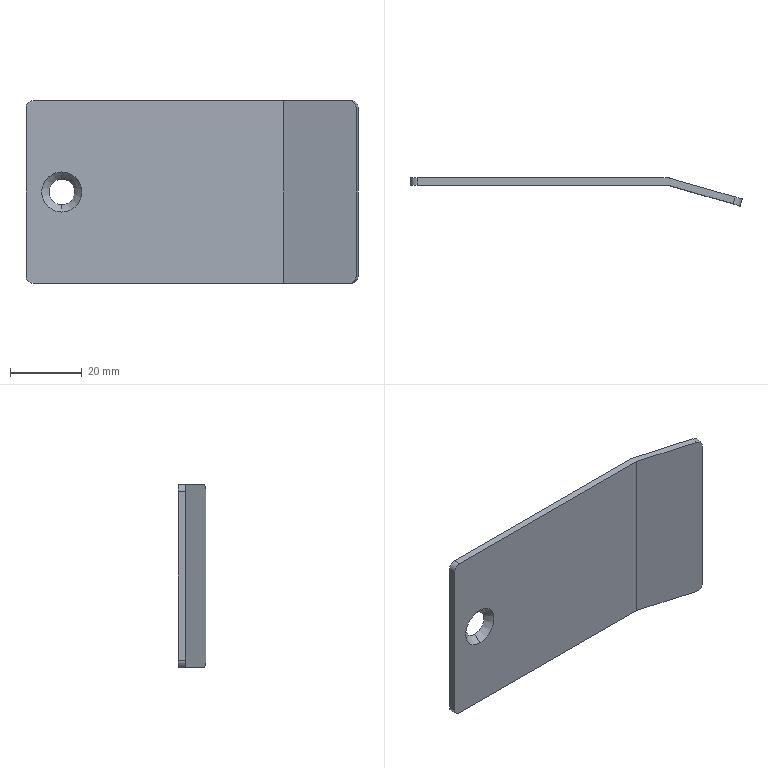Part | STEP file | Box cover | 1 solid | 15 faces | box 92.738 x 7.788 x 51 mm | volume 9373 mm3 | plane 8 | cylinder 5 | cone 2 | commonest cylinder face diameters 4 x4 3 x1
STEP:
#1=CARTESIAN_POINT('',(0.,0.,0.));
#2=DIRECTION('',(0.,0.,1.));
#3=DIRECTION('',(1.,0.,0.));
#4=AXIS2_PLACEMENT_3D('',#1,#2,#3);
#5=CARTESIAN_POINT('',(10.,2.,-3.6));
#6=VERTEX_POINT('',#5);
#7=CARTESIAN_POINT('',(10.,0.,-5.6));
#8=VERTEX_POINT('',#7);
#9=CARTESIAN_POINT('',(10.,0.,-5.6));
#10=DIRECTION('',(0.,-0.7071,-0.7071));
#11=VECTOR('',#10,1.);
#12=LINE('',#9,#11);
#13=CARTESIAN_POINT('',(10.,0.,0.));
#14=DIRECTION('',(0.,-1.,0.));
#15=DIRECTION('',(0.,0.,-1.));
#16=AXIS2_PLACEMENT_3D('',#13,#14,#15);
#17=CONICAL_SURFACE('',#16,5.6,0.7854);
#18=CARTESIAN_POINT('',(6.283,0.));
#19=DIRECTION('',(0.,1.));
#20=VECTOR('',#19,1.);
#21=LINE('',#18,#20);
#22=(GEOMETRIC_REPRESENTATION_CONTEXT(2)PARAMETRIC_REPRESENTATION_CONTEXT()REPRESENTATION_CONTEXT('',''));
#23=DEFINITIONAL_REPRESENTATION('',(#21),#22);
#24=PCURVE('',#17,#23);
#25=CARTESIAN_POINT('',(10.,0.,0.));
#26=DIRECTION('',(0.,-1.,0.));
#27=DIRECTION('',(0.,0.,-1.));
#28=AXIS2_PLACEMENT_3D('',#25,#26,#27);
#29=CONICAL_SURFACE('',#28,5.6,0.7854);
#30=CARTESIAN_POINT('',(0.,0.));
#31=DIRECTION('',(0.,1.));
#32=VECTOR('',#31,1.);
#33=LINE('',#30,#32);
#34=(GEOMETRIC_REPRESENTATION_CONTEXT(2)PARAMETRIC_REPRESENTATION_CONTEXT()REPRESENTATION_CONTEXT('',''));
#35=DEFINITIONAL_REPRESENTATION('',(#33),#34);
#36=PCURVE('',#29,#35);
#37=SURFACE_CURVE('',#12,(#24,#36),.PCURVE_S1.);
#38=EDGE_CURVE('',#6,#8,#37,.T.);
#39=ORIENTED_EDGE('',*,*,#38,.T.);
#40=CARTESIAN_POINT('',(10.,0.,5.6));
#41=VERTEX_POINT('',#40);
#42=CARTESIAN_POINT('',(10.,0.,0.));
#43=DIRECTION('',(0.,1.,0.));
#44=DIRECTION('',(0.,0.,-1.));
#45=AXIS2_PLACEMENT_3D('',#42,#43,#44);
#46=CIRCLE('',#45,5.6);
#47=CARTESIAN_POINT('',(6.283,0.));
#48=DIRECTION('',(-1.,0.));
#49=VECTOR('',#48,1.);
#50=LINE('',#47,#49);
#51=(GEOMETRIC_REPRESENTATION_CONTEXT(2)PARAMETRIC_REPRESENTATION_CONTEXT()REPRESENTATION_CONTEXT('',''));
#52=DEFINITIONAL_REPRESENTATION('',(#50),#51);
#53=PCURVE('',#17,#52);
#54=CARTESIAN_POINT('',(0.,0.,25.5));
#55=DIRECTION('',(0.,1.,0.));
#56=DIRECTION('',(0.,0.,1.));
#57=AXIS2_PLACEMENT_3D('',#54,#55,#56);
#58=PLANE('',#57);
#59=CARTESIAN_POINT('',(-25.5,10.));
#60=DIRECTION('',(-1.,0.));
#61=AXIS2_PLACEMENT_2D('',#59,#60);
#62=CIRCLE('',#61,5.6);
#63=(GEOMETRIC_REPRESENTATION_CONTEXT(2)PARAMETRIC_REPRESENTATION_CONTEXT()REPRESENTATION_CONTEXT('',''));
#64=DEFINITIONAL_REPRESENTATION('',(#62),#63);
#65=PCURVE('',#58,#64);
#66=SURFACE_CURVE('',#46,(#53,#65),.PCURVE_S1.);
#67=EDGE_CURVE('',#8,#41,#66,.T.);
#68=ORIENTED_EDGE('',*,*,#67,.T.);
#69=CARTESIAN_POINT('',(10.,2.,3.6));
#70=VERTEX_POINT('',#69);
#71=CARTESIAN_POINT('',(10.,0.,5.6));
#72=DIRECTION('',(0.,-0.7071,0.7071));
#73=VECTOR('',#72,1.);
#74=LINE('',#71,#73);
#75=CARTESIAN_POINT('',(3.142,0.));
#76=DIRECTION('',(0.,1.));
#77=VECTOR('',#76,1.);
#78=LINE('',#75,#77);
#79=(GEOMETRIC_REPRESENTATION_CONTEXT(2)PARAMETRIC_REPRESENTATION_CONTEXT()REPRESENTATION_CONTEXT('',''));
#80=DEFINITIONAL_REPRESENTATION('',(#78),#79);
#81=PCURVE('',#17,#80);
#82=CARTESIAN_POINT('',(3.142,0.));
#83=DIRECTION('',(0.,1.));
#84=VECTOR('',#83,1.);
#85=LINE('',#82,#84);
#86=(GEOMETRIC_REPRESENTATION_CONTEXT(2)PARAMETRIC_REPRESENTATION_CONTEXT()REPRESENTATION_CONTEXT('',''));
#87=DEFINITIONAL_REPRESENTATION('',(#85),#86);
#88=PCURVE('',#29,#87);
#89=SURFACE_CURVE('',#74,(#81,#88),.PCURVE_S1.);
#90=EDGE_CURVE('',#70,#41,#89,.T.);
#91=ORIENTED_EDGE('',*,*,#90,.F.);
#92=CARTESIAN_POINT('',(10.,2.,0.));
#93=DIRECTION('',(0.,-1.,0.));
#94=DIRECTION('',(0.,0.,-1.));
#95=AXIS2_PLACEMENT_3D('',#92,#93,#94);
#96=CIRCLE('',#95,3.6);
#97=CARTESIAN_POINT('',(0.,-2.));
#98=DIRECTION('',(1.,0.));
#99=VECTOR('',#98,1.);
#100=LINE('',#97,#99);
#101=(GEOMETRIC_REPRESENTATION_CONTEXT(2)PARAMETRIC_REPRESENTATION_CONTEXT()REPRESENTATION_CONTEXT('',''));
#102=DEFINITIONAL_REPRESENTATION('',(#100),#101);
#103=PCURVE('',#17,#102);
#104=CARTESIAN_POINT('',(0.,2.,25.5));
#105=DIRECTION('',(0.,1.,0.));
#106=DIRECTION('',(0.,0.,1.));
#107=AXIS2_PLACEMENT_3D('',#104,#105,#106);
#108=PLANE('',#107);
#109=CARTESIAN_POINT('',(-29.1,10.));
#110=CARTESIAN_POINT('',(-29.1,16.235));
#111=CARTESIAN_POINT('',(-23.7,13.118));
#112=CARTESIAN_POINT('',(-18.3,10.));
#113=CARTESIAN_POINT('',(-23.7,6.882));
#114=CARTESIAN_POINT('',(-29.1,3.765));
#115=CARTESIAN_POINT('',(-29.1,10.));
#116=(BOUNDED_CURVE()B_SPLINE_CURVE(2,(#109,#110,#111,#112,#113,#114,#115),.UNSPECIFIED.,.T.,.F.)B_SPLINE_CURVE_WITH_KNOTS((1,2,2,2,2,1),(-2.094,0.,2.094,4.189,6.283,8.378),.UNSPECIFIED.)CURVE()GEOMETRIC_REPRESENTATION_ITEM()RATIONAL_B_SPLINE_CURVE((1.,0.5,1.,0.5,1.,0.5,1.))REPRESENTATION_ITEM(''));
#117=(GEOMETRIC_REPRESENTATION_CONTEXT(2)PARAMETRIC_REPRESENTATION_CONTEXT()REPRESENTATION_CONTEXT('',''));
#118=DEFINITIONAL_REPRESENTATION('',(#116),#117);
#119=PCURVE('',#108,#118);
#120=SURFACE_CURVE('',#96,(#103,#119),.PCURVE_S1.);
#121=EDGE_CURVE('',#70,#6,#120,.T.);
#122=ORIENTED_EDGE('',*,*,#121,.T.);
#123=EDGE_LOOP('',(#39,#68,#91,#122));
#124=FACE_BOUND('',#123,.F.);
#125=ADVANCED_FACE('',(#124),#17,.F.);
#126=CARTESIAN_POINT('',(72.07,2.,-25.5));
#127=VERTEX_POINT('',#126);
#128=CARTESIAN_POINT('',(2.,2.,-25.5));
#129=VERTEX_POINT('',#128);
#130=CARTESIAN_POINT('',(0.,2.,-25.5));
#131=DIRECTION('',(-1.,0.,0.));
#132=VECTOR('',#131,1.);
#133=LINE('',#130,#132);
#134=CARTESIAN_POINT('',(-51.,0.));
#135=DIRECTION('',(0.,-1.));
#136=VECTOR('',#135,1.);
#137=LINE('',#134,#136);
#138=(GEOMETRIC_REPRESENTATION_CONTEXT(2)PARAMETRIC_REPRESENTATION_CONTEXT()REPRESENTATION_CONTEXT('',''));
#139=DEFINITIONAL_REPRESENTATION('',(#137),#138);
#140=PCURVE('',#108,#139);
#141=CARTESIAN_POINT('',(0.,2.,-25.5));
#142=DIRECTION('',(0.,0.,1.));
#143=DIRECTION('',(1.,0.,0.));
#144=AXIS2_PLACEMENT_3D('',#141,#142,#143);
#145=PLANE('',#144);
#146=CARTESIAN_POINT('',(0.,0.));
#147=DIRECTION('',(-1.,0.));
#148=VECTOR('',#147,1.);
#149=LINE('',#146,#148);
#150=(GEOMETRIC_REPRESENTATION_CONTEXT(2)PARAMETRIC_REPRESENTATION_CONTEXT()REPRESENTATION_CONTEXT('',''));
#151=DEFINITIONAL_REPRESENTATION('',(#149),#150);
#152=PCURVE('',#145,#151);
#153=SURFACE_CURVE('',#133,(#140,#152),.PCURVE_S1.);
#154=EDGE_CURVE('',#127,#129,#153,.T.);
#155=ORIENTED_EDGE('',*,*,#154,.T.);
#156=CARTESIAN_POINT('',(0.,2.,-23.5));
#157=VERTEX_POINT('',#156);
#158=CARTESIAN_POINT('',(2.,2.,-23.5));
#159=DIRECTION('',(0.,1.,0.));
#160=DIRECTION('',(0.,0.,-1.));
#161=AXIS2_PLACEMENT_3D('',#158,#159,#160);
#162=CIRCLE('',#161,2.);
#163=CARTESIAN_POINT('',(-49.,2.));
#164=DIRECTION('',(-1.,0.));
#165=AXIS2_PLACEMENT_2D('',#163,#164);
#166=CIRCLE('',#165,2.);
#167=(GEOMETRIC_REPRESENTATION_CONTEXT(2)PARAMETRIC_REPRESENTATION_CONTEXT()REPRESENTATION_CONTEXT('',''));
#168=DEFINITIONAL_REPRESENTATION('',(#166),#167);
#169=PCURVE('',#108,#168);
#170=CARTESIAN_POINT('',(2.,2.,-23.5));
#171=DIRECTION('',(0.,-1.,0.));
#172=DIRECTION('',(0.,0.,-1.));
#173=AXIS2_PLACEMENT_3D('',#170,#171,#172);
#174=CYLINDRICAL_SURFACE('',#173,2.);
#175=CARTESIAN_POINT('',(6.283,0.));
#176=DIRECTION('',(-1.,0.));
#177=VECTOR('',#176,1.);
#178=LINE('',#175,#177);
#179=(GEOMETRIC_REPRESENTATION_CONTEXT(2)PARAMETRIC_REPRESENTATION_CONTEXT()REPRESENTATION_CONTEXT('',''));
#180=DEFINITIONAL_REPRESENTATION('',(#178),#179);
#181=PCURVE('',#174,#180);
#182=SURFACE_CURVE('',#162,(#169,#181),.PCURVE_S1.);
#183=EDGE_CURVE('',#129,#157,#182,.T.);
#184=ORIENTED_EDGE('',*,*,#183,.T.);
#185=CARTESIAN_POINT('',(0.,2.,23.5));
#186=VERTEX_POINT('',#185);
#187=CARTESIAN_POINT('',(0.,2.,25.5));
#188=DIRECTION('',(0.,0.,1.));
#189=VECTOR('',#188,1.);
#190=LINE('',#187,#189);
#191=CARTESIAN_POINT('',(0.,0.));
#192=DIRECTION('',(1.,0.));
#193=VECTOR('',#192,1.);
#194=LINE('',#191,#193);
#195=(GEOMETRIC_REPRESENTATION_CONTEXT(2)PARAMETRIC_REPRESENTATION_CONTEXT()REPRESENTATION_CONTEXT('',''));
#196=DEFINITIONAL_REPRESENTATION('',(#194),#195);
#197=PCURVE('',#108,#196);
#198=CARTESIAN_POINT('',(0.,2.,-25.5));
#199=DIRECTION('',(1.,0.,0.));
#200=DIRECTION('',(0.,0.,-1.));
#201=AXIS2_PLACEMENT_3D('',#198,#199,#200);
#202=PLANE('',#201);
#203=CARTESIAN_POINT('',(-51.,0.));
#204=DIRECTION('',(-1.,0.));
#205=VECTOR('',#204,1.);
#206=LINE('',#203,#205);
#207=(GEOMETRIC_REPRESENTATION_CONTEXT(2)PARAMETRIC_REPRESENTATION_CONTEXT()REPRESENTATION_CONTEXT('',''));
#208=DEFINITIONAL_REPRESENTATION('',(#206),#207);
#209=PCURVE('',#202,#208);
#210=SURFACE_CURVE('',#190,(#197,#209),.PCURVE_S1.);
#211=EDGE_CURVE('',#157,#186,#210,.T.);
#212=ORIENTED_EDGE('',*,*,#211,.T.);
#213=CARTESIAN_POINT('',(2.,2.,25.5));
#214=VERTEX_POINT('',#213);
#215=CARTESIAN_POINT('',(2.,2.,23.5));
#216=DIRECTION('',(0.,1.,0.));
#217=DIRECTION('',(0.,0.,-1.));
#218=AXIS2_PLACEMENT_3D('',#215,#216,#217);
#219=CIRCLE('',#218,2.);
#220=CARTESIAN_POINT('',(-2.,2.));
#221=DIRECTION('',(-1.,0.));
#222=AXIS2_PLACEMENT_2D('',#220,#221);
#223=CIRCLE('',#222,2.);
#224=(GEOMETRIC_REPRESENTATION_CONTEXT(2)PARAMETRIC_REPRESENTATION_CONTEXT()REPRESENTATION_CONTEXT('',''));
#225=DEFINITIONAL_REPRESENTATION('',(#223),#224);
#226=PCURVE('',#108,#225);
#227=CARTESIAN_POINT('',(2.,2.,23.5));
#228=DIRECTION('',(0.,-1.,0.));
#229=DIRECTION('',(0.,0.,-1.));
#230=AXIS2_PLACEMENT_3D('',#227,#228,#229);
#231=CYLINDRICAL_SURFACE('',#230,2.);
#232=CARTESIAN_POINT('',(6.283,0.));
#233=DIRECTION('',(-1.,0.));
#234=VECTOR('',#233,1.);
#235=LINE('',#232,#234);
#236=(GEOMETRIC_REPRESENTATION_CONTEXT(2)PARAMETRIC_REPRESENTATION_CONTEXT()REPRESENTATION_CONTEXT('',''));
#237=DEFINITIONAL_REPRESENTATION('',(#235),#236);
#238=PCURVE('',#231,#237);
#239=SURFACE_CURVE('',#219,(#226,#238),.PCURVE_S1.);
#240=EDGE_CURVE('',#186,#214,#239,.T.);
#241=ORIENTED_EDGE('',*,*,#240,.T.);
#242=CARTESIAN_POINT('',(72.07,2.,25.5));
#243=VERTEX_POINT('',#242);
#244=CARTESIAN_POINT('',(0.,2.,25.5));
#245=DIRECTION('',(1.,0.,0.));
#246=VECTOR('',#245,1.);
#247=LINE('',#244,#246);
#248=CARTESIAN_POINT('',(0.,0.));
#249=DIRECTION('',(0.,1.));
#250=VECTOR('',#249,1.);
#251=LINE('',#248,#250);
#252=(GEOMETRIC_REPRESENTATION_CONTEXT(2)PARAMETRIC_REPRESENTATION_CONTEXT()REPRESENTATION_CONTEXT('',''));
#253=DEFINITIONAL_REPRESENTATION('',(#251),#252);
#254=PCURVE('',#108,#253);
#255=CARTESIAN_POINT('',(0.,2.,25.5));
#256=DIRECTION('',(0.,0.,-1.));
#257=DIRECTION('',(-1.,0.,0.));
#258=AXIS2_PLACEMENT_3D('',#255,#256,#257);
#259=PLANE('',#258);
#260=CARTESIAN_POINT('',(0.,0.));
#261=DIRECTION('',(-1.,0.));
#262=VECTOR('',#261,1.);
#263=LINE('',#260,#262);
#264=(GEOMETRIC_REPRESENTATION_CONTEXT(2)PARAMETRIC_REPRESENTATION_CONTEXT()REPRESENTATION_CONTEXT('',''));
#265=DEFINITIONAL_REPRESENTATION('',(#263),#264);
#266=PCURVE('',#259,#265);
#267=SURFACE_CURVE('',#247,(#254,#266),.PCURVE_S1.);
#268=EDGE_CURVE('',#214,#243,#267,.T.);
#269=ORIENTED_EDGE('',*,*,#268,.T.);
#270=CARTESIAN_POINT('',(72.07,2.,25.5));
#271=DIRECTION('',(0.,0.,-1.));
#272=VECTOR('',#271,1.);
#273=LINE('',#270,#272);
#274=CARTESIAN_POINT('',(0.,72.07));
#275=DIRECTION('',(-1.,0.));
#276=VECTOR('',#275,1.);
#277=LINE('',#274,#276);
#278=(GEOMETRIC_REPRESENTATION_CONTEXT(2)PARAMETRIC_REPRESENTATION_CONTEXT()REPRESENTATION_CONTEXT('',''));
#279=DEFINITIONAL_REPRESENTATION('',(#277),#278);
#280=PCURVE('',#108,#279);
#281=CARTESIAN_POINT('',(72.07,0.5,-47.652));
#282=DIRECTION('',(0.,0.,1.));
#283=DIRECTION('',(1.,0.,0.));
#284=AXIS2_PLACEMENT_3D('',#281,#282,#283);
#285=CYLINDRICAL_SURFACE('',#284,1.5);
#286=CARTESIAN_POINT('',(1.571,73.152));
#287=DIRECTION('',(0.,-1.));
#288=VECTOR('',#287,1.);
#289=LINE('',#286,#288);
#290=(GEOMETRIC_REPRESENTATION_CONTEXT(2)PARAMETRIC_REPRESENTATION_CONTEXT()REPRESENTATION_CONTEXT('',''));
#291=DEFINITIONAL_REPRESENTATION('',(#289),#290);
#292=PCURVE('',#285,#291);
#293=SURFACE_CURVE('',#273,(#280,#292),.PCURVE_S1.);
#294=EDGE_CURVE('',#243,#127,#293,.T.);
#295=ORIENTED_EDGE('',*,*,#294,.T.);
#296=EDGE_LOOP('',(#155,#184,#212,#241,#269,#295));
#297=FACE_BOUND('',#296,.T.);
#298=CARTESIAN_POINT('',(10.,2.,0.));
#299=DIRECTION('',(0.,-1.,0.));
#300=DIRECTION('',(0.,0.,-1.));
#301=AXIS2_PLACEMENT_3D('',#298,#299,#300);
#302=CIRCLE('',#301,3.6);
#303=CARTESIAN_POINT('',(-29.1,10.));
#304=CARTESIAN_POINT('',(-29.1,16.235));
#305=CARTESIAN_POINT('',(-23.7,13.118));
#306=CARTESIAN_POINT('',(-18.3,10.));
#307=CARTESIAN_POINT('',(-23.7,6.882));
#308=CARTESIAN_POINT('',(-29.1,3.765));
#309=CARTESIAN_POINT('',(-29.1,10.));
#310=(BOUNDED_CURVE()B_SPLINE_CURVE(2,(#303,#304,#305,#306,#307,#308,#309),.UNSPECIFIED.,.T.,.F.)B_SPLINE_CURVE_WITH_KNOTS((1,2,2,2,2,1),(-2.094,0.,2.094,4.189,6.283,8.378),.UNSPECIFIED.)CURVE()GEOMETRIC_REPRESENTATION_ITEM()RATIONAL_B_SPLINE_CURVE((1.,0.5,1.,0.5,1.,0.5,1.))REPRESENTATION_ITEM(''));
#311=(GEOMETRIC_REPRESENTATION_CONTEXT(2)PARAMETRIC_REPRESENTATION_CONTEXT()REPRESENTATION_CONTEXT('',''));
#312=DEFINITIONAL_REPRESENTATION('',(#310),#311);
#313=PCURVE('',#108,#312);
#314=CARTESIAN_POINT('',(0.,-2.));
#315=DIRECTION('',(1.,0.));
#316=VECTOR('',#315,1.);
#317=LINE('',#314,#316);
#318=(GEOMETRIC_REPRESENTATION_CONTEXT(2)PARAMETRIC_REPRESENTATION_CONTEXT()REPRESENTATION_CONTEXT('',''));
#319=DEFINITIONAL_REPRESENTATION('',(#317),#318);
#320=PCURVE('',#29,#319);
#321=SURFACE_CURVE('',#302,(#313,#320),.PCURVE_S1.);
#322=EDGE_CURVE('',#6,#70,#321,.T.);
#323=ORIENTED_EDGE('',*,*,#322,.T.);
#324=ORIENTED_EDGE('',*,*,#121,.T.);
#325=EDGE_LOOP('',(#323,#324));
#326=FACE_BOUND('',#325,.T.);
#327=ADVANCED_FACE('',(#297,#326),#108,.T.);
#328=CARTESIAN_POINT('',(2.,0.,-25.5));
#329=VERTEX_POINT('',#328);
#330=CARTESIAN_POINT('',(0.,0.,-23.5));
#331=VERTEX_POINT('',#330);
#332=CARTESIAN_POINT('',(2.,0.,-23.5));
#333=DIRECTION('',(0.,1.,0.));
#334=DIRECTION('',(0.,0.,-1.));
#335=AXIS2_PLACEMENT_3D('',#332,#333,#334);
#336=CIRCLE('',#335,2.);
#337=CARTESIAN_POINT('',(6.283,2.));
#338=DIRECTION('',(-1.,0.));
#339=VECTOR('',#338,1.);
#340=LINE('',#337,#339);
#341=(GEOMETRIC_REPRESENTATION_CONTEXT(2)PARAMETRIC_REPRESENTATION_CONTEXT()REPRESENTATION_CONTEXT('',''));
#342=DEFINITIONAL_REPRESENTATION('',(#340),#341);
#343=PCURVE('',#174,#342);
#344=CARTESIAN_POINT('',(-49.,2.));
#345=DIRECTION('',(-1.,0.));
#346=AXIS2_PLACEMENT_2D('',#344,#345);
#347=CIRCLE('',#346,2.);
#348=(GEOMETRIC_REPRESENTATION_CONTEXT(2)PARAMETRIC_REPRESENTATION_CONTEXT()REPRESENTATION_CONTEXT('',''));
#349=DEFINITIONAL_REPRESENTATION('',(#347),#348);
#350=PCURVE('',#58,#349);
#351=SURFACE_CURVE('',#336,(#343,#350),.PCURVE_S1.);
#352=EDGE_CURVE('',#329,#331,#351,.T.);
#353=ORIENTED_EDGE('',*,*,#352,.T.);
#354=CARTESIAN_POINT('',(0.,2.,-23.5));
#355=DIRECTION('',(0.,1.,0.));
#356=VECTOR('',#355,1.);
#357=LINE('',#354,#356);
#358=CARTESIAN_POINT('',(4.712,0.));
#359=DIRECTION('',(0.,-1.));
#360=VECTOR('',#359,1.);
#361=LINE('',#358,#360);
#362=(GEOMETRIC_REPRESENTATION_CONTEXT(2)PARAMETRIC_REPRESENTATION_CONTEXT()REPRESENTATION_CONTEXT('',''));
#363=DEFINITIONAL_REPRESENTATION('',(#361),#362);
#364=PCURVE('',#174,#363);
#365=CARTESIAN_POINT('',(-2.,0.));
#366=DIRECTION('',(0.,1.));
#367=VECTOR('',#366,1.);
#368=LINE('',#365,#367);
#369=(GEOMETRIC_REPRESENTATION_CONTEXT(2)PARAMETRIC_REPRESENTATION_CONTEXT()REPRESENTATION_CONTEXT('',''));
#370=DEFINITIONAL_REPRESENTATION('',(#368),#369);
#371=PCURVE('',#202,#370);
#372=SURFACE_CURVE('',#357,(#364,#371),.PCURVE_S1.);
#373=EDGE_CURVE('',#331,#157,#372,.T.);
#374=ORIENTED_EDGE('',*,*,#373,.T.);
#375=ORIENTED_EDGE('',*,*,#183,.F.);
#376=CARTESIAN_POINT('',(2.,2.,-25.5));
#377=DIRECTION('',(0.,-1.,0.));
#378=VECTOR('',#377,1.);
#379=LINE('',#376,#378);
#380=CARTESIAN_POINT('',(6.283,0.));
#381=DIRECTION('',(0.,1.));
#382=VECTOR('',#381,1.);
#383=LINE('',#380,#382);
#384=(GEOMETRIC_REPRESENTATION_CONTEXT(2)PARAMETRIC_REPRESENTATION_CONTEXT()REPRESENTATION_CONTEXT('',''));
#385=DEFINITIONAL_REPRESENTATION('',(#383),#384);
#386=PCURVE('',#174,#385);
#387=CARTESIAN_POINT('',(2.,0.));
#388=DIRECTION('',(0.,-1.));
#389=VECTOR('',#388,1.);
#390=LINE('',#387,#389);
#391=(GEOMETRIC_REPRESENTATION_CONTEXT(2)PARAMETRIC_REPRESENTATION_CONTEXT()REPRESENTATION_CONTEXT('',''));
#392=DEFINITIONAL_REPRESENTATION('',(#390),#391);
#393=PCURVE('',#145,#392);
#394=SURFACE_CURVE('',#379,(#386,#393),.PCURVE_S1.);
#395=EDGE_CURVE('',#129,#329,#394,.T.);
#396=ORIENTED_EDGE('',*,*,#395,.T.);
#397=EDGE_LOOP('',(#353,#374,#375,#396));
#398=FACE_BOUND('',#397,.T.);
#399=ADVANCED_FACE('',(#398),#174,.T.);
#400=ORIENTED_EDGE('',*,*,#395,.F.);
#401=ORIENTED_EDGE('',*,*,#154,.F.);
#402=CARTESIAN_POINT('',(72.484,1.942,-25.5));
#403=VERTEX_POINT('',#402);
#404=CARTESIAN_POINT('',(72.07,0.5,-25.5));
#405=DIRECTION('',(0.,0.,1.));
#406=DIRECTION('',(1.,0.,0.));
#407=AXIS2_PLACEMENT_3D('',#404,#405,#406);
#408=CIRCLE('',#407,1.5);
#409=CARTESIAN_POINT('',(72.07,-1.5));
#410=DIRECTION('',(1.,0.));
#411=AXIS2_PLACEMENT_2D('',#409,#410);
#412=CIRCLE('',#411,1.5);
#413=(GEOMETRIC_REPRESENTATION_CONTEXT(2)PARAMETRIC_REPRESENTATION_CONTEXT()REPRESENTATION_CONTEXT('',''));
#414=DEFINITIONAL_REPRESENTATION('',(#412),#413);
#415=PCURVE('',#145,#414);
#416=CARTESIAN_POINT('',(0.,22.152));
#417=DIRECTION('',(1.,0.));
#418=VECTOR('',#417,1.);
#419=LINE('',#416,#418);
#420=(GEOMETRIC_REPRESENTATION_CONTEXT(2)PARAMETRIC_REPRESENTATION_CONTEXT()REPRESENTATION_CONTEXT('',''));
#421=DEFINITIONAL_REPRESENTATION('',(#419),#420);
#422=PCURVE('',#285,#421);
#423=SURFACE_CURVE('',#408,(#415,#422),.PCURVE_S1.);
#424=EDGE_CURVE('',#403,#127,#423,.T.);
#425=ORIENTED_EDGE('',*,*,#424,.F.);
#426=CARTESIAN_POINT('',(90.815,-3.315,-25.5));
#427=VERTEX_POINT('',#426);
#428=CARTESIAN_POINT('',(90.815,-3.315,-25.5));
#429=DIRECTION('',(-0.9613,0.2756,0.));
#430=VECTOR('',#429,1.);
#431=LINE('',#428,#430);
#432=CARTESIAN_POINT('',(90.815,-5.315));
#433=DIRECTION('',(-0.9613,0.2756));
#434=VECTOR('',#433,1.);
#435=LINE('',#432,#434);
#436=(GEOMETRIC_REPRESENTATION_CONTEXT(2)PARAMETRIC_REPRESENTATION_CONTEXT()REPRESENTATION_CONTEXT('',''));
#437=DEFINITIONAL_REPRESENTATION('',(#435),#436);
#438=PCURVE('',#145,#437);
#439=CARTESIAN_POINT('',(72.484,1.942,-47.652));
#440=DIRECTION('',(0.2756,0.9613,0.));
#441=DIRECTION('',(-0.9613,0.2756,0.));
#442=AXIS2_PLACEMENT_3D('',#439,#440,#441);
#443=PLANE('',#442);
#444=CARTESIAN_POINT('',(-19.07,22.152));
#445=DIRECTION('',(1.,0.));
#446=VECTOR('',#445,1.);
#447=LINE('',#444,#446);
#448=(GEOMETRIC_REPRESENTATION_CONTEXT(2)PARAMETRIC_REPRESENTATION_CONTEXT()REPRESENTATION_CONTEXT('',''));
#449=DEFINITIONAL_REPRESENTATION('',(#447),#448);
#450=PCURVE('',#443,#449);
#451=SURFACE_CURVE('',#431,(#438,#450),.PCURVE_S1.);
#452=EDGE_CURVE('',#427,#403,#451,.T.);
#453=ORIENTED_EDGE('',*,*,#452,.F.);
#454=CARTESIAN_POINT('',(90.264,-5.237,-25.5));
#455=VERTEX_POINT('',#454);
#456=CARTESIAN_POINT('',(90.264,-5.237,-25.5));
#457=DIRECTION('',(0.2756,0.9613,0.));
#458=VECTOR('',#457,1.);
#459=LINE('',#456,#458);
#460=CARTESIAN_POINT('',(90.264,-7.237));
#461=DIRECTION('',(0.2756,0.9613));
#462=VECTOR('',#461,1.);
#463=LINE('',#460,#462);
#464=(GEOMETRIC_REPRESENTATION_CONTEXT(2)PARAMETRIC_REPRESENTATION_CONTEXT()REPRESENTATION_CONTEXT('',''));
#465=DEFINITIONAL_REPRESENTATION('',(#463),#464);
#466=PCURVE('',#145,#465);
#467=CARTESIAN_POINT('',(85.324,-22.466,-23.5));
#468=DIRECTION('',(0.2756,0.9613,0.));
#469=DIRECTION('',(-0.9613,0.2756,0.));
#470=AXIS2_PLACEMENT_3D('',#467,#468,#469);
#471=CYLINDRICAL_SURFACE('',#470,2.);
#472=CARTESIAN_POINT('',(4.712,17.923));
#473=DIRECTION('',(0.,1.));
#474=VECTOR('',#473,1.);
#475=LINE('',#472,#474);
#476=(GEOMETRIC_REPRESENTATION_CONTEXT(2)PARAMETRIC_REPRESENTATION_CONTEXT()REPRESENTATION_CONTEXT('',''));
#477=DEFINITIONAL_REPRESENTATION('',(#475),#476);
#478=PCURVE('',#471,#477);
#479=SURFACE_CURVE('',#459,(#466,#478),.PCURVE_S1.);
#480=EDGE_CURVE('',#455,#427,#479,.T.);
#481=ORIENTED_EDGE('',*,*,#480,.F.);
#482=CARTESIAN_POINT('',(72.,0.,-25.5));
#483=VERTEX_POINT('',#482);
#484=CARTESIAN_POINT('',(72.,0.,-25.5));
#485=DIRECTION('',(0.9613,-0.2756,0.));
#486=VECTOR('',#485,1.);
#487=LINE('',#484,#486);
#488=CARTESIAN_POINT('',(72.,-2.));
#489=DIRECTION('',(0.9613,-0.2756));
#490=VECTOR('',#489,1.);
#491=LINE('',#488,#490);
#492=(GEOMETRIC_REPRESENTATION_CONTEXT(2)PARAMETRIC_REPRESENTATION_CONTEXT()REPRESENTATION_CONTEXT('',''));
#493=DEFINITIONAL_REPRESENTATION('',(#491),#492);
#494=PCURVE('',#145,#493);
#495=CARTESIAN_POINT('',(72.,0.,-47.652));
#496=DIRECTION('',(-0.2756,-0.9613,0.));
#497=DIRECTION('',(0.9613,-0.2756,0.));
#498=AXIS2_PLACEMENT_3D('',#495,#496,#497);
#499=PLANE('',#498);
#500=CARTESIAN_POINT('',(0.,22.152));
#501=DIRECTION('',(1.,0.));
#502=VECTOR('',#501,1.);
#503=LINE('',#500,#502);
#504=(GEOMETRIC_REPRESENTATION_CONTEXT(2)PARAMETRIC_REPRESENTATION_CONTEXT()REPRESENTATION_CONTEXT('',''));
#505=DEFINITIONAL_REPRESENTATION('',(#503),#504);
#506=PCURVE('',#499,#505);
#507=SURFACE_CURVE('',#487,(#494,#506),.PCURVE_S1.);
#508=EDGE_CURVE('',#483,#455,#507,.T.);
#509=ORIENTED_EDGE('',*,*,#508,.F.);
#510=CARTESIAN_POINT('',(0.,0.,-25.5));
#511=DIRECTION('',(1.,0.,0.));
#512=VECTOR('',#511,1.);
#513=LINE('',#510,#512);
#514=CARTESIAN_POINT('',(0.,-2.));
#515=DIRECTION('',(1.,0.));
#516=VECTOR('',#515,1.);
#517=LINE('',#514,#516);
#518=(GEOMETRIC_REPRESENTATION_CONTEXT(2)PARAMETRIC_REPRESENTATION_CONTEXT()REPRESENTATION_CONTEXT('',''));
#519=DEFINITIONAL_REPRESENTATION('',(#517),#518);
#520=PCURVE('',#145,#519);
#521=CARTESIAN_POINT('',(-51.,0.));
#522=DIRECTION('',(0.,1.));
#523=VECTOR('',#522,1.);
#524=LINE('',#521,#523);
#525=(GEOMETRIC_REPRESENTATION_CONTEXT(2)PARAMETRIC_REPRESENTATION_CONTEXT()REPRESENTATION_CONTEXT('',''));
#526=DEFINITIONAL_REPRESENTATION('',(#524),#525);
#527=PCURVE('',#58,#526);
#528=SURFACE_CURVE('',#513,(#520,#527),.PCURVE_S1.);
#529=EDGE_CURVE('',#329,#483,#528,.T.);
#530=ORIENTED_EDGE('',*,*,#529,.F.);
#531=EDGE_LOOP('',(#400,#401,#425,#453,#481,#509,#530));
#532=FACE_BOUND('',#531,.T.);
#533=ADVANCED_FACE('',(#532),#145,.F.);
#534=CARTESIAN_POINT('',(72.484,1.942,25.5));
#535=VERTEX_POINT('',#534);
#536=CARTESIAN_POINT('',(72.07,0.5,25.5));
#537=DIRECTION('',(0.,0.,-1.));
#538=DIRECTION('',(1.,0.,0.));
#539=AXIS2_PLACEMENT_3D('',#536,#537,#538);
#540=CIRCLE('',#539,1.5);
#541=CARTESIAN_POINT('',(6.283,73.152));
#542=DIRECTION('',(-1.,0.));
#543=VECTOR('',#542,1.);
#544=LINE('',#541,#543);
#545=(GEOMETRIC_REPRESENTATION_CONTEXT(2)PARAMETRIC_REPRESENTATION_CONTEXT()REPRESENTATION_CONTEXT('',''));
#546=DEFINITIONAL_REPRESENTATION('',(#544),#545);
#547=PCURVE('',#285,#546);
#548=CARTESIAN_POINT('',(-72.07,-1.5));
#549=DIRECTION('',(-1.,0.));
#550=AXIS2_PLACEMENT_2D('',#548,#549);
#551=CIRCLE('',#550,1.5);
#552=(GEOMETRIC_REPRESENTATION_CONTEXT(2)PARAMETRIC_REPRESENTATION_CONTEXT()REPRESENTATION_CONTEXT('',''));
#553=DEFINITIONAL_REPRESENTATION('',(#551),#552);
#554=PCURVE('',#259,#553);
#555=SURFACE_CURVE('',#540,(#547,#554),.PCURVE_S1.);
#556=EDGE_CURVE('',#243,#535,#555,.T.);
#557=ORIENTED_EDGE('',*,*,#556,.T.);
#558=CARTESIAN_POINT('',(72.484,1.942,-47.652));
#559=DIRECTION('',(0.,0.,-1.));
#560=VECTOR('',#559,1.);
#561=LINE('',#558,#560);
#562=CARTESIAN_POINT('',(1.292,0.));
#563=DIRECTION('',(0.,-1.));
#564=VECTOR('',#563,1.);
#565=LINE('',#562,#564);
#566=(GEOMETRIC_REPRESENTATION_CONTEXT(2)PARAMETRIC_REPRESENTATION_CONTEXT()REPRESENTATION_CONTEXT('',''));
#567=DEFINITIONAL_REPRESENTATION('',(#565),#566);
#568=PCURVE('',#285,#567);
#569=CARTESIAN_POINT('',(0.,0.));
#570=DIRECTION('',(0.,-1.));
#571=VECTOR('',#570,1.);
#572=LINE('',#569,#571);
#573=(GEOMETRIC_REPRESENTATION_CONTEXT(2)PARAMETRIC_REPRESENTATION_CONTEXT()REPRESENTATION_CONTEXT('',''));
#574=DEFINITIONAL_REPRESENTATION('',(#572),#573);
#575=PCURVE('',#443,#574);
#576=SURFACE_CURVE('',#561,(#568,#575),.PCURVE_S1.);
#577=EDGE_CURVE('',#535,#403,#576,.T.);
#578=ORIENTED_EDGE('',*,*,#577,.T.);
#579=ORIENTED_EDGE('',*,*,#424,.T.);
#580=ORIENTED_EDGE('',*,*,#294,.F.);
#581=EDGE_LOOP('',(#557,#578,#579,#580));
#582=FACE_BOUND('',#581,.T.);
#583=ADVANCED_FACE('',(#582),#285,.T.);
#584=CARTESIAN_POINT('',(2.,0.,25.5));
#585=VERTEX_POINT('',#584);
#586=CARTESIAN_POINT('',(2.,2.,25.5));
#587=DIRECTION('',(0.,1.,0.));
#588=VECTOR('',#587,1.);
#589=LINE('',#586,#588);
#590=CARTESIAN_POINT('',(-2.,0.));
#591=DIRECTION('',(0.,1.));
#592=VECTOR('',#591,1.);
#593=LINE('',#590,#592);
#594=(GEOMETRIC_REPRESENTATION_CONTEXT(2)PARAMETRIC_REPRESENTATION_CONTEXT()REPRESENTATION_CONTEXT('',''));
#595=DEFINITIONAL_REPRESENTATION('',(#593),#594);
#596=PCURVE('',#259,#595);
#597=CARTESIAN_POINT('',(3.142,0.));
#598=DIRECTION('',(0.,-1.));
#599=VECTOR('',#598,1.);
#600=LINE('',#597,#599);
#601=(GEOMETRIC_REPRESENTATION_CONTEXT(2)PARAMETRIC_REPRESENTATION_CONTEXT()REPRESENTATION_CONTEXT('',''));
#602=DEFINITIONAL_REPRESENTATION('',(#600),#601);
#603=PCURVE('',#231,#602);
#604=SURFACE_CURVE('',#589,(#596,#603),.PCURVE_S1.);
#605=EDGE_CURVE('',#585,#214,#604,.T.);
#606=ORIENTED_EDGE('',*,*,#605,.F.);
#607=CARTESIAN_POINT('',(72.,0.,25.5));
#608=VERTEX_POINT('',#607);
#609=CARTESIAN_POINT('',(0.,0.,25.5));
#610=DIRECTION('',(-1.,0.,0.));
#611=VECTOR('',#610,1.);
#612=LINE('',#609,#611);
#613=CARTESIAN_POINT('',(0.,-2.));
#614=DIRECTION('',(1.,0.));
#615=VECTOR('',#614,1.);
#616=LINE('',#613,#615);
#617=(GEOMETRIC_REPRESENTATION_CONTEXT(2)PARAMETRIC_REPRESENTATION_CONTEXT()REPRESENTATION_CONTEXT('',''));
#618=DEFINITIONAL_REPRESENTATION('',(#616),#617);
#619=PCURVE('',#259,#618);
#620=CARTESIAN_POINT('',(0.,0.));
#621=DIRECTION('',(0.,-1.));
#622=VECTOR('',#621,1.);
#623=LINE('',#620,#622);
#624=(GEOMETRIC_REPRESENTATION_CONTEXT(2)PARAMETRIC_REPRESENTATION_CONTEXT()REPRESENTATION_CONTEXT('',''));
#625=DEFINITIONAL_REPRESENTATION('',(#623),#624);
#626=PCURVE('',#58,#625);
#627=SURFACE_CURVE('',#612,(#619,#626),.PCURVE_S1.);
#628=EDGE_CURVE('',#608,#585,#627,.T.);
#629=ORIENTED_EDGE('',*,*,#628,.F.);
#630=CARTESIAN_POINT('',(90.264,-5.237,25.5));
#631=VERTEX_POINT('',#630);
#632=CARTESIAN_POINT('',(90.264,-5.237,25.5));
#633=DIRECTION('',(-0.9613,0.2756,0.));
#634=VECTOR('',#633,1.);
#635=LINE('',#632,#634);
#636=CARTESIAN_POINT('',(-90.264,-7.237));
#637=DIRECTION('',(0.9613,0.2756));
#638=VECTOR('',#637,1.);
#639=LINE('',#636,#638);
#640=(GEOMETRIC_REPRESENTATION_CONTEXT(2)PARAMETRIC_REPRESENTATION_CONTEXT()REPRESENTATION_CONTEXT('',''));
#641=DEFINITIONAL_REPRESENTATION('',(#639),#640);
#642=PCURVE('',#259,#641);
#643=CARTESIAN_POINT('',(19.,73.152));
#644=DIRECTION('',(-1.,0.));
#645=VECTOR('',#644,1.);
#646=LINE('',#643,#645);
#647=(GEOMETRIC_REPRESENTATION_CONTEXT(2)PARAMETRIC_REPRESENTATION_CONTEXT()REPRESENTATION_CONTEXT('',''));
#648=DEFINITIONAL_REPRESENTATION('',(#646),#647);
#649=PCURVE('',#499,#648);
#650=SURFACE_CURVE('',#635,(#642,#649),.PCURVE_S1.);
#651=EDGE_CURVE('',#631,#608,#650,.T.);
#652=ORIENTED_EDGE('',*,*,#651,.F.);
#653=CARTESIAN_POINT('',(90.815,-3.315,25.5));
#654=VERTEX_POINT('',#653);
#655=CARTESIAN_POINT('',(90.815,-3.315,25.5));
#656=DIRECTION('',(-0.2756,-0.9613,0.));
#657=VECTOR('',#656,1.);
#658=LINE('',#655,#657);
#659=CARTESIAN_POINT('',(-90.815,-5.315));
#660=DIRECTION('',(0.2756,-0.9613));
#661=VECTOR('',#660,1.);
#662=LINE('',#659,#661);
#663=(GEOMETRIC_REPRESENTATION_CONTEXT(2)PARAMETRIC_REPRESENTATION_CONTEXT()REPRESENTATION_CONTEXT('',''));
#664=DEFINITIONAL_REPRESENTATION('',(#662),#663);
#665=PCURVE('',#259,#664);
#666=CARTESIAN_POINT('',(85.324,-22.466,23.5));
#667=DIRECTION('',(-0.2756,-0.9613,0.));
#668=DIRECTION('',(0.9613,-0.2756,0.));
#669=AXIS2_PLACEMENT_3D('',#666,#667,#668);
#670=CYLINDRICAL_SURFACE('',#669,2.);
#671=CARTESIAN_POINT('',(1.571,-19.923));
#672=DIRECTION('',(0.,1.));
#673=VECTOR('',#672,1.);
#674=LINE('',#671,#673);
#675=(GEOMETRIC_REPRESENTATION_CONTEXT(2)PARAMETRIC_REPRESENTATION_CONTEXT()REPRESENTATION_CONTEXT('',''));
#676=DEFINITIONAL_REPRESENTATION('',(#674),#675);
#677=PCURVE('',#670,#676);
#678=SURFACE_CURVE('',#658,(#665,#677),.PCURVE_S1.);
#679=EDGE_CURVE('',#654,#631,#678,.T.);
#680=ORIENTED_EDGE('',*,*,#679,.F.);
#681=CARTESIAN_POINT('',(72.484,1.942,25.5));
#682=DIRECTION('',(0.9613,-0.2756,0.));
#683=VECTOR('',#682,1.);
#684=LINE('',#681,#683);
#685=CARTESIAN_POINT('',(-72.484,-0.05811));
#686=DIRECTION('',(-0.9613,-0.2756));
#687=VECTOR('',#686,1.);
#688=LINE('',#685,#687);
#689=(GEOMETRIC_REPRESENTATION_CONTEXT(2)PARAMETRIC_REPRESENTATION_CONTEXT()REPRESENTATION_CONTEXT('',''));
#690=DEFINITIONAL_REPRESENTATION('',(#688),#689);
#691=PCURVE('',#259,#690);
#692=CARTESIAN_POINT('',(0.,73.152));
#693=DIRECTION('',(-1.,0.));
#694=VECTOR('',#693,1.);
#695=LINE('',#692,#694);
#696=(GEOMETRIC_REPRESENTATION_CONTEXT(2)PARAMETRIC_REPRESENTATION_CONTEXT()REPRESENTATION_CONTEXT('',''));
#697=DEFINITIONAL_REPRESENTATION('',(#695),#696);
#698=PCURVE('',#443,#697);
#699=SURFACE_CURVE('',#684,(#691,#698),.PCURVE_S1.);
#700=EDGE_CURVE('',#535,#654,#699,.T.);
#701=ORIENTED_EDGE('',*,*,#700,.F.);
#702=ORIENTED_EDGE('',*,*,#556,.F.);
#703=ORIENTED_EDGE('',*,*,#268,.F.);
#704=EDGE_LOOP('',(#606,#629,#652,#680,#701,#702,#703));
#705=FACE_BOUND('',#704,.T.);
#706=ADVANCED_FACE('',(#705),#259,.F.);
#707=CARTESIAN_POINT('',(0.,0.,23.5));
#708=VERTEX_POINT('',#707);
#709=CARTESIAN_POINT('',(2.,0.,23.5));
#710=DIRECTION('',(0.,1.,0.));
#711=DIRECTION('',(0.,0.,-1.));
#712=AXIS2_PLACEMENT_3D('',#709,#710,#711);
#713=CIRCLE('',#712,2.);
#714=CARTESIAN_POINT('',(6.283,2.));
#715=DIRECTION('',(-1.,0.));
#716=VECTOR('',#715,1.);
#717=LINE('',#714,#716);
#718=(GEOMETRIC_REPRESENTATION_CONTEXT(2)PARAMETRIC_REPRESENTATION_CONTEXT()REPRESENTATION_CONTEXT('',''));
#719=DEFINITIONAL_REPRESENTATION('',(#717),#718);
#720=PCURVE('',#231,#719);
#721=CARTESIAN_POINT('',(-2.,2.));
#722=DIRECTION('',(-1.,0.));
#723=AXIS2_PLACEMENT_2D('',#721,#722);
#724=CIRCLE('',#723,2.);
#725=(GEOMETRIC_REPRESENTATION_CONTEXT(2)PARAMETRIC_REPRESENTATION_CONTEXT()REPRESENTATION_CONTEXT('',''));
#726=DEFINITIONAL_REPRESENTATION('',(#724),#725);
#727=PCURVE('',#58,#726);
#728=SURFACE_CURVE('',#713,(#720,#727),.PCURVE_S1.);
#729=EDGE_CURVE('',#708,#585,#728,.T.);
#730=ORIENTED_EDGE('',*,*,#729,.T.);
#731=ORIENTED_EDGE('',*,*,#605,.T.);
#732=ORIENTED_EDGE('',*,*,#240,.F.);
#733=CARTESIAN_POINT('',(0.,2.,23.5));
#734=DIRECTION('',(0.,-1.,0.));
#735=VECTOR('',#734,1.);
#736=LINE('',#733,#735);
#737=CARTESIAN_POINT('',(4.712,0.));
#738=DIRECTION('',(0.,1.));
#739=VECTOR('',#738,1.);
#740=LINE('',#737,#739);
#741=(GEOMETRIC_REPRESENTATION_CONTEXT(2)PARAMETRIC_REPRESENTATION_CONTEXT()REPRESENTATION_CONTEXT('',''));
#742=DEFINITIONAL_REPRESENTATION('',(#740),#741);
#743=PCURVE('',#231,#742);
#744=CARTESIAN_POINT('',(-49.,0.));
#745=DIRECTION('',(0.,-1.));
#746=VECTOR('',#745,1.);
#747=LINE('',#744,#746);
#748=(GEOMETRIC_REPRESENTATION_CONTEXT(2)PARAMETRIC_REPRESENTATION_CONTEXT()REPRESENTATION_CONTEXT('',''));
#749=DEFINITIONAL_REPRESENTATION('',(#747),#748);
#750=PCURVE('',#202,#749);
#751=SURFACE_CURVE('',#736,(#743,#750),.PCURVE_S1.);
#752=EDGE_CURVE('',#186,#708,#751,.T.);
#753=ORIENTED_EDGE('',*,*,#752,.T.);
#754=EDGE_LOOP('',(#730,#731,#732,#753));
#755=FACE_BOUND('',#754,.T.);
#756=ADVANCED_FACE('',(#755),#231,.T.);
#757=ORIENTED_EDGE('',*,*,#752,.F.);
#758=ORIENTED_EDGE('',*,*,#211,.F.);
#759=ORIENTED_EDGE('',*,*,#373,.F.);
#760=CARTESIAN_POINT('',(0.,0.,-25.5));
#761=DIRECTION('',(0.,0.,-1.));
#762=VECTOR('',#761,1.);
#763=LINE('',#760,#762);
#764=CARTESIAN_POINT('',(0.,-2.));
#765=DIRECTION('',(1.,0.));
#766=VECTOR('',#765,1.);
#767=LINE('',#764,#766);
#768=(GEOMETRIC_REPRESENTATION_CONTEXT(2)PARAMETRIC_REPRESENTATION_CONTEXT()REPRESENTATION_CONTEXT('',''));
#769=DEFINITIONAL_REPRESENTATION('',(#767),#768);
#770=PCURVE('',#202,#769);
#771=CARTESIAN_POINT('',(-51.,0.));
#772=DIRECTION('',(-1.,0.));
#773=VECTOR('',#772,1.);
#774=LINE('',#771,#773);
#775=(GEOMETRIC_REPRESENTATION_CONTEXT(2)PARAMETRIC_REPRESENTATION_CONTEXT()REPRESENTATION_CONTEXT('',''));
#776=DEFINITIONAL_REPRESENTATION('',(#774),#775);
#777=PCURVE('',#58,#776);
#778=SURFACE_CURVE('',#763,(#770,#777),.PCURVE_S1.);
#779=EDGE_CURVE('',#708,#331,#778,.T.);
#780=ORIENTED_EDGE('',*,*,#779,.F.);
#781=EDGE_LOOP('',(#757,#758,#759,#780));
#782=FACE_BOUND('',#781,.T.);
#783=ADVANCED_FACE('',(#782),#202,.F.);
#784=CARTESIAN_POINT('',(10.,0.,0.));
#785=DIRECTION('',(0.,1.,0.));
#786=DIRECTION('',(0.,0.,-1.));
#787=AXIS2_PLACEMENT_3D('',#784,#785,#786);
#788=CIRCLE('',#787,5.6);
#789=CARTESIAN_POINT('',(6.283,0.));
#790=DIRECTION('',(-1.,0.));
#791=VECTOR('',#790,1.);
#792=LINE('',#789,#791);
#793=(GEOMETRIC_REPRESENTATION_CONTEXT(2)PARAMETRIC_REPRESENTATION_CONTEXT()REPRESENTATION_CONTEXT('',''));
#794=DEFINITIONAL_REPRESENTATION('',(#792),#793);
#795=PCURVE('',#29,#794);
#796=CARTESIAN_POINT('',(-25.5,10.));
#797=DIRECTION('',(-1.,0.));
#798=AXIS2_PLACEMENT_2D('',#796,#797);
#799=CIRCLE('',#798,5.6);
#800=(GEOMETRIC_REPRESENTATION_CONTEXT(2)PARAMETRIC_REPRESENTATION_CONTEXT()REPRESENTATION_CONTEXT('',''));
#801=DEFINITIONAL_REPRESENTATION('',(#799),#800);
#802=PCURVE('',#58,#801);
#803=SURFACE_CURVE('',#788,(#795,#802),.PCURVE_S1.);
#804=EDGE_CURVE('',#41,#8,#803,.T.);
#805=ORIENTED_EDGE('',*,*,#804,.T.);
#806=ORIENTED_EDGE('',*,*,#38,.F.);
#807=ORIENTED_EDGE('',*,*,#322,.T.);
#808=ORIENTED_EDGE('',*,*,#90,.T.);
#809=EDGE_LOOP('',(#805,#806,#807,#808));
#810=FACE_BOUND('',#809,.F.);
#811=ADVANCED_FACE('',(#810),#29,.F.);
#812=ORIENTED_EDGE('',*,*,#729,.F.);
#813=ORIENTED_EDGE('',*,*,#779,.T.);
#814=ORIENTED_EDGE('',*,*,#352,.F.);
#815=ORIENTED_EDGE('',*,*,#529,.T.);
#816=CARTESIAN_POINT('',(72.,0.,25.5));
#817=DIRECTION('',(0.,0.,-1.));
#818=VECTOR('',#817,1.);
#819=LINE('',#816,#818);
#820=CARTESIAN_POINT('',(0.,72.));
#821=DIRECTION('',(-1.,0.));
#822=VECTOR('',#821,1.);
#823=LINE('',#820,#822);
#824=(GEOMETRIC_REPRESENTATION_CONTEXT(2)PARAMETRIC_REPRESENTATION_CONTEXT()REPRESENTATION_CONTEXT('',''));
#825=DEFINITIONAL_REPRESENTATION('',(#823),#824);
#826=PCURVE('',#58,#825);
#827=CARTESIAN_POINT('',(0.,73.152));
#828=DIRECTION('',(0.,-1.));
#829=VECTOR('',#828,1.);
#830=LINE('',#827,#829);
#831=(GEOMETRIC_REPRESENTATION_CONTEXT(2)PARAMETRIC_REPRESENTATION_CONTEXT()REPRESENTATION_CONTEXT('',''));
#832=DEFINITIONAL_REPRESENTATION('',(#830),#831);
#833=PCURVE('',#499,#832);
#834=SURFACE_CURVE('',#819,(#826,#833),.PCURVE_S1.);
#835=EDGE_CURVE('',#608,#483,#834,.T.);
#836=ORIENTED_EDGE('',*,*,#835,.F.);
#837=ORIENTED_EDGE('',*,*,#628,.T.);
#838=EDGE_LOOP('',(#812,#813,#814,#815,#836,#837));
#839=FACE_BOUND('',#838,.T.);
#840=ORIENTED_EDGE('',*,*,#67,.T.);
#841=ORIENTED_EDGE('',*,*,#804,.T.);
#842=EDGE_LOOP('',(#840,#841));
#843=FACE_BOUND('',#842,.T.);
#844=ADVANCED_FACE('',(#839,#843),#58,.F.);
#845=ORIENTED_EDGE('',*,*,#700,.T.);
#846=CARTESIAN_POINT('',(92.738,-3.866,23.5));
#847=VERTEX_POINT('',#846);
#848=CARTESIAN_POINT('',(90.815,-3.315,23.5));
#849=DIRECTION('',(0.2756,0.9613,0.));
#850=DIRECTION('',(0.9613,-0.2756,0.));
#851=AXIS2_PLACEMENT_3D('',#848,#849,#850);
#852=CIRCLE('',#851,2.);
#853=CARTESIAN_POINT('',(-19.07,71.152));
#854=DIRECTION('',(-1.,0.));
#855=AXIS2_PLACEMENT_2D('',#853,#854);
#856=CIRCLE('',#855,2.);
#857=(GEOMETRIC_REPRESENTATION_CONTEXT(2)PARAMETRIC_REPRESENTATION_CONTEXT()REPRESENTATION_CONTEXT('',''));
#858=DEFINITIONAL_REPRESENTATION('',(#856),#857);
#859=PCURVE('',#443,#858);
#860=CARTESIAN_POINT('',(6.283,-19.923));
#861=DIRECTION('',(-1.,0.));
#862=VECTOR('',#861,1.);
#863=LINE('',#860,#862);
#864=(GEOMETRIC_REPRESENTATION_CONTEXT(2)PARAMETRIC_REPRESENTATION_CONTEXT()REPRESENTATION_CONTEXT('',''));
#865=DEFINITIONAL_REPRESENTATION('',(#863),#864);
#866=PCURVE('',#670,#865);
#867=SURFACE_CURVE('',#852,(#859,#866),.PCURVE_S1.);
#868=EDGE_CURVE('',#654,#847,#867,.T.);
#869=ORIENTED_EDGE('',*,*,#868,.T.);
#870=CARTESIAN_POINT('',(92.738,-3.866,-23.5));
#871=VERTEX_POINT('',#870);
#872=CARTESIAN_POINT('',(92.738,-3.866,-47.652));
#873=DIRECTION('',(0.,0.,-1.));
#874=VECTOR('',#873,1.);
#875=LINE('',#872,#874);
#876=CARTESIAN_POINT('',(-21.07,0.));
#877=DIRECTION('',(0.,-1.));
#878=VECTOR('',#877,1.);
#879=LINE('',#876,#878);
#880=(GEOMETRIC_REPRESENTATION_CONTEXT(2)PARAMETRIC_REPRESENTATION_CONTEXT()REPRESENTATION_CONTEXT('',''));
#881=DEFINITIONAL_REPRESENTATION('',(#879),#880);
#882=PCURVE('',#443,#881);
#883=CARTESIAN_POINT('',(92.186,-5.788,-47.652));
#884=DIRECTION('',(0.9613,-0.2756,0.));
#885=DIRECTION('',(0.2756,0.9613,0.));
#886=AXIS2_PLACEMENT_3D('',#883,#884,#885);
#887=PLANE('',#886);
#888=CARTESIAN_POINT('',(2.,0.));
#889=DIRECTION('',(0.,-1.));
#890=VECTOR('',#889,1.);
#891=LINE('',#888,#890);
#892=(GEOMETRIC_REPRESENTATION_CONTEXT(2)PARAMETRIC_REPRESENTATION_CONTEXT()REPRESENTATION_CONTEXT('',''));
#893=DEFINITIONAL_REPRESENTATION('',(#891),#892);
#894=PCURVE('',#887,#893);
#895=SURFACE_CURVE('',#875,(#882,#894),.PCURVE_S1.);
#896=EDGE_CURVE('',#847,#871,#895,.T.);
#897=ORIENTED_EDGE('',*,*,#896,.T.);
#898=CARTESIAN_POINT('',(90.815,-3.315,-23.5));
#899=DIRECTION('',(0.2756,0.9613,0.));
#900=DIRECTION('',(-0.9613,0.2756,0.));
#901=AXIS2_PLACEMENT_3D('',#898,#899,#900);
#902=CIRCLE('',#901,2.);
#903=CARTESIAN_POINT('',(-19.07,24.152));
#904=DIRECTION('',(1.,0.));
#905=AXIS2_PLACEMENT_2D('',#903,#904);
#906=CIRCLE('',#905,2.);
#907=(GEOMETRIC_REPRESENTATION_CONTEXT(2)PARAMETRIC_REPRESENTATION_CONTEXT()REPRESENTATION_CONTEXT('',''));
#908=DEFINITIONAL_REPRESENTATION('',(#906),#907);
#909=PCURVE('',#443,#908);
#910=CARTESIAN_POINT('',(0.,19.923));
#911=DIRECTION('',(1.,0.));
#912=VECTOR('',#911,1.);
#913=LINE('',#910,#912);
#914=(GEOMETRIC_REPRESENTATION_CONTEXT(2)PARAMETRIC_REPRESENTATION_CONTEXT()REPRESENTATION_CONTEXT('',''));
#915=DEFINITIONAL_REPRESENTATION('',(#913),#914);
#916=PCURVE('',#471,#915);
#917=SURFACE_CURVE('',#902,(#909,#916),.PCURVE_S1.);
#918=EDGE_CURVE('',#871,#427,#917,.T.);
#919=ORIENTED_EDGE('',*,*,#918,.T.);
#920=ORIENTED_EDGE('',*,*,#452,.T.);
#921=ORIENTED_EDGE('',*,*,#577,.F.);
#922=EDGE_LOOP('',(#845,#869,#897,#919,#920,#921));
#923=FACE_BOUND('',#922,.T.);
#924=ADVANCED_FACE('',(#923),#443,.T.);
#925=CARTESIAN_POINT('',(92.186,-5.788,-23.5));
#926=VERTEX_POINT('',#925);
#927=CARTESIAN_POINT('',(90.264,-5.237,-23.5));
#928=DIRECTION('',(0.2756,0.9613,0.));
#929=DIRECTION('',(-0.9613,0.2756,0.));
#930=AXIS2_PLACEMENT_3D('',#927,#928,#929);
#931=CIRCLE('',#930,2.);
#932=CARTESIAN_POINT('',(0.,17.923));
#933=DIRECTION('',(1.,0.));
#934=VECTOR('',#933,1.);
#935=LINE('',#932,#934);
#936=(GEOMETRIC_REPRESENTATION_CONTEXT(2)PARAMETRIC_REPRESENTATION_CONTEXT()REPRESENTATION_CONTEXT('',''));
#937=DEFINITIONAL_REPRESENTATION('',(#935),#936);
#938=PCURVE('',#471,#937);
#939=CARTESIAN_POINT('',(17.,24.152));
#940=CARTESIAN_POINT('',(17.,27.616));
#941=CARTESIAN_POINT('',(20.,25.884));
#942=CARTESIAN_POINT('',(23.,24.152));
#943=CARTESIAN_POINT('',(20.,22.42));
#944=CARTESIAN_POINT('',(17.,20.688));
#945=CARTESIAN_POINT('',(17.,24.152));
#946=(BOUNDED_CURVE()B_SPLINE_CURVE(2,(#939,#940,#941,#942,#943,#944,#945),.UNSPECIFIED.,.T.,.F.)B_SPLINE_CURVE_WITH_KNOTS((1,2,2,2,2,1),(-2.094,0.,2.094,4.189,6.283,8.378),.UNSPECIFIED.)CURVE()GEOMETRIC_REPRESENTATION_ITEM()RATIONAL_B_SPLINE_CURVE((1.,0.5,1.,0.5,1.,0.5,1.))REPRESENTATION_ITEM(''));
#947=(GEOMETRIC_REPRESENTATION_CONTEXT(2)PARAMETRIC_REPRESENTATION_CONTEXT()REPRESENTATION_CONTEXT('',''));
#948=DEFINITIONAL_REPRESENTATION('',(#946),#947);
#949=PCURVE('',#499,#948);
#950=SURFACE_CURVE('',#931,(#938,#949),.PCURVE_S1.);
#951=EDGE_CURVE('',#926,#455,#950,.T.);
#952=ORIENTED_EDGE('',*,*,#951,.T.);
#953=ORIENTED_EDGE('',*,*,#480,.T.);
#954=ORIENTED_EDGE('',*,*,#918,.F.);
#955=CARTESIAN_POINT('',(87.246,-23.017,-23.5));
#956=DIRECTION('',(-0.2756,-0.9613,0.));
#957=VECTOR('',#956,1.);
#958=LINE('',#955,#957);
#959=CARTESIAN_POINT('',(3.142,0.));
#960=DIRECTION('',(0.,-1.));
#961=VECTOR('',#960,1.);
#962=LINE('',#959,#961);
#963=(GEOMETRIC_REPRESENTATION_CONTEXT(2)PARAMETRIC_REPRESENTATION_CONTEXT()REPRESENTATION_CONTEXT('',''));
#964=DEFINITIONAL_REPRESENTATION('',(#962),#963);
#965=PCURVE('',#471,#964);
#966=CARTESIAN_POINT('',(-17.923,24.152));
#967=DIRECTION('',(-1.,0.));
#968=VECTOR('',#967,1.);
#969=LINE('',#966,#968);
#970=(GEOMETRIC_REPRESENTATION_CONTEXT(2)PARAMETRIC_REPRESENTATION_CONTEXT()REPRESENTATION_CONTEXT('',''));
#971=DEFINITIONAL_REPRESENTATION('',(#969),#970);
#972=PCURVE('',#887,#971);
#973=SURFACE_CURVE('',#958,(#965,#972),.PCURVE_S1.);
#974=EDGE_CURVE('',#871,#926,#973,.T.);
#975=ORIENTED_EDGE('',*,*,#974,.T.);
#976=EDGE_LOOP('',(#952,#953,#954,#975));
#977=FACE_BOUND('',#976,.T.);
#978=ADVANCED_FACE('',(#977),#471,.T.);
#979=ORIENTED_EDGE('',*,*,#651,.T.);
#980=ORIENTED_EDGE('',*,*,#835,.T.);
#981=ORIENTED_EDGE('',*,*,#508,.T.);
#982=ORIENTED_EDGE('',*,*,#951,.F.);
#983=CARTESIAN_POINT('',(92.186,-5.788,23.5));
#984=VERTEX_POINT('',#983);
#985=CARTESIAN_POINT('',(92.186,-5.788,-47.652));
#986=DIRECTION('',(0.,0.,1.));
#987=VECTOR('',#986,1.);
#988=LINE('',#985,#987);
#989=CARTESIAN_POINT('',(21.,0.));
#990=DIRECTION('',(0.,1.));
#991=VECTOR('',#990,1.);
#992=LINE('',#989,#991);
#993=(GEOMETRIC_REPRESENTATION_CONTEXT(2)PARAMETRIC_REPRESENTATION_CONTEXT()REPRESENTATION_CONTEXT('',''));
#994=DEFINITIONAL_REPRESENTATION('',(#992),#993);
#995=PCURVE('',#499,#994);
#996=CARTESIAN_POINT('',(0.,0.));
#997=DIRECTION('',(0.,1.));
#998=VECTOR('',#997,1.);
#999=LINE('',#996,#998);
#1000=(GEOMETRIC_REPRESENTATION_CONTEXT(2)PARAMETRIC_REPRESENTATION_CONTEXT()REPRESENTATION_CONTEXT('',''));
#1001=DEFINITIONAL_REPRESENTATION('',(#999),#1000);
#1002=PCURVE('',#887,#1001);
#1003=SURFACE_CURVE('',#988,(#995,#1002),.PCURVE_S1.);
#1004=EDGE_CURVE('',#926,#984,#1003,.T.);
#1005=ORIENTED_EDGE('',*,*,#1004,.T.);
#1006=CARTESIAN_POINT('',(90.264,-5.237,23.5));
#1007=DIRECTION('',(-0.2756,-0.9613,0.));
#1008=DIRECTION('',(0.9613,-0.2756,0.));
#1009=AXIS2_PLACEMENT_3D('',#1006,#1007,#1008);
#1010=CIRCLE('',#1009,2.);
#1011=CARTESIAN_POINT('',(19.,71.152));
#1012=DIRECTION('',(1.,0.));
#1013=AXIS2_PLACEMENT_2D('',#1011,#1012);
#1014=CIRCLE('',#1013,2.);
#1015=(GEOMETRIC_REPRESENTATION_CONTEXT(2)PARAMETRIC_REPRESENTATION_CONTEXT()REPRESENTATION_CONTEXT('',''));
#1016=DEFINITIONAL_REPRESENTATION('',(#1014),#1015);
#1017=PCURVE('',#499,#1016);
#1018=CARTESIAN_POINT('',(0.,-17.923));
#1019=DIRECTION('',(1.,0.));
#1020=VECTOR('',#1019,1.);
#1021=LINE('',#1018,#1020);
#1022=(GEOMETRIC_REPRESENTATION_CONTEXT(2)PARAMETRIC_REPRESENTATION_CONTEXT()REPRESENTATION_CONTEXT('',''));
#1023=DEFINITIONAL_REPRESENTATION('',(#1021),#1022);
#1024=PCURVE('',#670,#1023);
#1025=SURFACE_CURVE('',#1010,(#1017,#1024),.PCURVE_S1.);
#1026=EDGE_CURVE('',#984,#631,#1025,.T.);
#1027=ORIENTED_EDGE('',*,*,#1026,.T.);
#1028=EDGE_LOOP('',(#979,#980,#981,#982,#1005,#1027));
#1029=FACE_BOUND('',#1028,.T.);
#1030=ADVANCED_FACE('',(#1029),#499,.T.);
#1031=ORIENTED_EDGE('',*,*,#868,.F.);
#1032=ORIENTED_EDGE('',*,*,#679,.T.);
#1033=ORIENTED_EDGE('',*,*,#1026,.F.);
#1034=CARTESIAN_POINT('',(87.246,-23.017,23.5));
#1035=DIRECTION('',(0.2756,0.9613,0.));
#1036=VECTOR('',#1035,1.);
#1037=LINE('',#1034,#1036);
#1038=CARTESIAN_POINT('',(0.,0.));
#1039=DIRECTION('',(0.,-1.));
#1040=VECTOR('',#1039,1.);
#1041=LINE('',#1038,#1040);
#1042=(GEOMETRIC_REPRESENTATION_CONTEXT(2)PARAMETRIC_REPRESENTATION_CONTEXT()REPRESENTATION_CONTEXT('',''));
#1043=DEFINITIONAL_REPRESENTATION('',(#1041),#1042);
#1044=PCURVE('',#670,#1043);
#1045=CARTESIAN_POINT('',(-17.923,71.152));
#1046=DIRECTION('',(1.,0.));
#1047=VECTOR('',#1046,1.);
#1048=LINE('',#1045,#1047);
#1049=(GEOMETRIC_REPRESENTATION_CONTEXT(2)PARAMETRIC_REPRESENTATION_CONTEXT()REPRESENTATION_CONTEXT('',''));
#1050=DEFINITIONAL_REPRESENTATION('',(#1048),#1049);
#1051=PCURVE('',#887,#1050);
#1052=SURFACE_CURVE('',#1037,(#1044,#1051),.PCURVE_S1.);
#1053=EDGE_CURVE('',#984,#847,#1052,.T.);
#1054=ORIENTED_EDGE('',*,*,#1053,.T.);
#1055=EDGE_LOOP('',(#1031,#1032,#1033,#1054));
#1056=FACE_BOUND('',#1055,.T.);
#1057=ADVANCED_FACE('',(#1056),#670,.T.);
#1058=ORIENTED_EDGE('',*,*,#896,.F.);
#1059=ORIENTED_EDGE('',*,*,#1053,.F.);
#1060=ORIENTED_EDGE('',*,*,#1004,.F.);
#1061=ORIENTED_EDGE('',*,*,#974,.F.);
#1062=EDGE_LOOP('',(#1058,#1059,#1060,#1061));
#1063=FACE_BOUND('',#1062,.T.);
#1064=ADVANCED_FACE('',(#1063),#887,.T.);
#1065=CLOSED_SHELL('',(#125,#327,#399,#533,#583,#706,#756,#783,#811,#844,#924,#978,#1030,#1057,#1064));
#1066=MANIFOLD_SOLID_BREP('',#1065);
#1067=(LENGTH_UNIT()NAMED_UNIT(*)SI_UNIT(.MILLI.,.METRE.));
#1068=UNCERTAINTY_MEASURE_WITH_UNIT(LENGTH_MEASURE(0.0000001),#1067,'','');
#1069=(NAMED_UNIT(*)PLANE_ANGLE_UNIT()SI_UNIT($,.RADIAN.));
#1070=(NAMED_UNIT(*)SI_UNIT($,.STERADIAN.)SOLID_ANGLE_UNIT());
#1071=(GEOMETRIC_REPRESENTATION_CONTEXT(3)GLOBAL_UNCERTAINTY_ASSIGNED_CONTEXT((#1068))GLOBAL_UNIT_ASSIGNED_CONTEXT((#1067,#1069,#1070))REPRESENTATION_CONTEXT('',''));
#1072=ADVANCED_BREP_SHAPE_REPRESENTATION('',(#4,#1066),#1071);